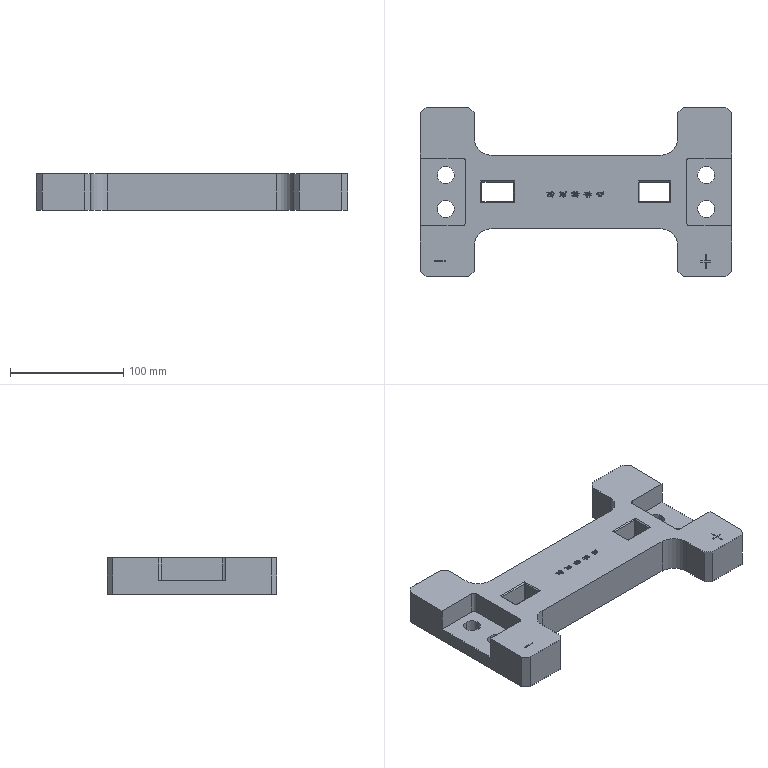NC program | NX | posted with a generic post | part box 275 x 150 x 32 mm
Lines 9668 to 10049 of 10049:
(DRILLING_COPY_1_COPY_1 , TOOL : ZXZ)
N19328 T01 M6
N19330 G54
N19332 G17 G0 G90 X-115. Y-15. S5000 M3
N19334 G43 Z30. H1
N19336 G94 G81 G98 Z-20.8 F250. R-16.8
N19338 Y15.
N19340 X-69.5 Y0. Z-1. R3.
N19342 X69.5
N19344 X115. Y15. Z-20.8 R-16.8
N19346 Y-15.
N19348 G80
N19350 G0 X115. Y-15. Z30.
N19352 M5
(FLOOR_WALL_1_1_COPY , TOOL : D10JING)
N19354 T11 M6
N19356 G54
N19358 G17 G0 G90 X-143. Y-23.634 S7000 M3
N19360 G43 Z30. H11
N19362 Z-18.8
N19364 G94 G1 Z-19.8 F1000.
N19366 X-142.
N19368 G3 X-142.5 Y-24.5 R1.
N19370 G1 Y24.5
N19372 X-137.562
N19374 Y-24.5
N19376 X-132.625
N19378 Y24.5
N19380 X-127.687
N19382 Y-24.5
N19384 X-122.75
N19386 Y24.5
N19388 X-117.813
N19390 Y-24.5
N19392 X-112.875
N19394 Y24.5
N19396 X-107.938
N19398 Y-24.5
N19400 X-103.
N19402 Y24.5
N19404 G3 X-103.25 Y24.433 R0.5
N19406 G1 Z-18.8
N19408 G0 Z30.
N19410 X-143.366 Y-24.5
N19412 Z-18.8
N19414 G1 Z-19.8
N19416 G3 X-142.5 Y-25. R1.
N19418 G1 X-102.5
N19420 Y25.
N19422 X-142.5
N19424 G3 X-143.366 Y24.5 R1.
N19426 G1 Z-18.8
N19428 G0 Z30.
N19430 X143. Y23.634
N19432 Z-18.8
N19434 G1 Z-19.8
N19436 X142.
N19438 G3 X142.5 Y24.5 R1.
N19440 G1 Y-24.5
N19442 X137.562
N19444 Y24.5
N19446 X132.625
N19448 Y-24.5
N19450 X127.687
N19452 Y24.5
N19454 X122.75
N19456 Y-24.5
N19458 X117.813
N19460 Y24.5
N19462 X112.875
N19464 Y-24.5
N19466 X107.938
N19468 Y24.5
N19470 X103.
N19472 Y-24.5
N19474 G3 X103.25 Y-24.433 R0.5
N19476 G1 Z-18.8
N19478 G0 Z30.
N19480 X143.366 Y24.5
N19482 Z-18.8
N19484 G1 Z-19.8
N19486 G3 X142.5 Y25. R1.
N19488 G1 X102.5
N19490 Y-25.
N19492 X142.5
N19494 G3 X143.366 Y-24.5 R1.
N19496 G1 Z-18.8
N19498 G0 Z30.
(ZLEVEL_PROFILE_1_COPY_COPY , TOOL : D10JING)
N19500 X-136.193 Y-81.161 S7500
N19502 Z-14.925
N19504 G1 Z-15.925 F1250.
N19506 X-135.527 Y-80.211
N19508 G3 X-135.639 Y-78.93 R1.
N19510 G1 X-138.3 Y-76.271
N19512 X-141.036 Y-73.536
N19514 X-141.43 Y-73.139
N19516 G3 X-142.711 Y-73.024 R1.
N19518 G1 X-143.665 Y-73.688
N19520 Z-14.925
N19522 G0 Z30.
N19524 X-136.194 Y-81.164
N19526 Z-30.85
N19528 G1 Z-31.85
N19530 X-135.528 Y-80.212
N19532 G3 X-135.64 Y-78.931 R1.
N19534 G1 X-138.3 Y-76.271
N19536 X-141.036 Y-73.536
N19538 X-141.431 Y-73.14
N19540 G3 X-142.712 Y-73.027 R1.
N19542 G1 X-143.664 Y-73.694
N19544 Z-30.85
N19546 G0 Z30.
N19548 X-143.662 Y73.693
N19550 Z-14.925
N19552 G1 Z-15.925
N19554 X-142.711 Y73.027
N19556 G3 X-141.43 Y73.139 R1.
N19558 G1 X-139.64 Y74.931
N19560 X-136.036 Y78.536
N19562 X-135.639 Y78.93
N19564 G3 X-135.524 Y80.211 R1.
N19566 G1 X-136.188 Y81.165
N19568 Z-14.925
N19570 G0 Z30.
N19572 X-143.664 Y73.694
N19574 Z-30.85
N19576 G1 Z-31.85
N19578 X-142.712 Y73.028
N19580 G3 X-141.431 Y73.14 R1.
N19582 G1 X-139.64 Y74.931
N19584 X-136.036 Y78.536
N19586 X-135.64 Y78.931
N19588 G3 X-135.527 Y80.212 R1.
N19590 G1 X-136.194 Y81.164
N19592 Z-30.85
N19594 G0 Z30.
N19596 X-91.669 Y81.429
N19598 Z-14.925
N19600 G1 Z-15.925
N19602 X-92.296 Y80.53
N19604 G3 X-92.181 Y79.249 R1.
N19606 G1 X-91.49 Y78.561
N19608 X-87.043 Y74.114
N19610 X-86.994 Y74.073
N19612 X-87.039 Y74.029
N19614 G2 X-85. Y70. R5.
N19616 G1 Y47.5
N19618 G3 X-75. Y37.5 R10.
N19620 G1 X75.
N19622 G3 X85. Y47.5 R10.
N19624 G1 Y70.
N19626 G2 X86.891 Y73.916 R5.
N19628 G1 X86.907 Y73.971
N19630 X87.172 Y74.243
N19632 X91.464 Y78.536
N19634 X92.181 Y79.249
N19636 G3 X92.296 Y80.53 R1.
N19638 G1 X91.672 Y81.425
N19640 Z-14.925
N19642 G0 Z30.
N19644 X-91.665 Y81.428
N19646 Z-30.85
N19648 G1 Z-31.85
N19650 X-92.293 Y80.532
N19652 G3 X-92.18 Y79.251 R1.
N19654 G1 X-91.49 Y78.561
N19656 X-87.042 Y74.113
N19658 X-86.994 Y74.073
N19660 X-87.039 Y74.029
N19662 G2 X-85. Y70. R5.
N19664 G1 Y47.5
N19666 G3 X-75. Y37.5 R10.
N19668 G1 X75.
N19670 G3 X85. Y47.5 R10.
N19672 G1 Y70.
N19674 G2 X86.891 Y73.916 R5.
N19676 G1 X86.906 Y73.972
N19678 X87.172 Y74.243
N19680 X91.464 Y78.536
N19682 X92.18 Y79.251
N19684 G3 X92.293 Y80.532 R1.
N19686 G1 X91.668 Y81.424
N19688 Z-30.85
N19690 G0 Z30.
N19692 X91.665 Y-81.426
N19694 Z-14.925
N19696 G1 Z-15.925
N19698 X92.293 Y-80.53
N19700 G3 X92.181 Y-79.249 R1.
N19702 G1 X89.77 Y-76.841
N19704 X86.464 Y-73.536
N19706 G2 X85. Y-70. R5.
N19708 G1 Y-47.5
N19710 G3 X75. Y-37.5 R10.
N19712 G1 X-75.
N19714 G3 X-85. Y-47.5 R10.
N19716 G1 Y-70.
N19718 G2 X-86.464 Y-73.536 R5.
N19720 G1 X-89.804 Y-76.871
N19722 X-92.181 Y-79.249
N19724 G3 X-92.293 Y-80.53 R1.
N19726 G1 X-91.668 Y-81.422
N19728 Z-14.925
N19730 G0 Z30.
N19732 X91.665 Y-81.428
N19734 Z-30.85
N19736 G1 Z-31.85
N19738 X92.292 Y-80.532
N19740 G3 X92.18 Y-79.251 R1.
N19742 G1 X89.77 Y-76.841
N19744 X86.464 Y-73.536
N19746 G2 X85. Y-70. R5.
N19748 G1 Y-47.5
N19750 G3 X75. Y-37.5 R10.
N19752 G1 X-75.
N19754 G3 X-85. Y-47.5 R10.
N19756 G1 Y-70.
N19758 G2 X-86.464 Y-73.536 R5.
N19760 G1 X-89.77 Y-76.841
N19762 X-92.18 Y-79.251
N19764 G3 X-92.292 Y-80.532 R1.
N19766 G1 X-91.668 Y-81.424
N19768 Z-30.85
N19770 G0 Z30.
N19772 X143.919 Y-73.34
N19774 Z-14.925
N19776 G1 Z-15.925
N19778 X143.02 Y-72.713
N19780 G3 X141.74 Y-72.828 R1.
N19782 G1 X141.06 Y-73.511
N19784 X138.273 Y-76.294
N19786 X135.639 Y-78.93
N19788 G3 X135.527 Y-80.211 R1.
N19790 G1 X136.193 Y-81.161
N19792 Z-14.925
N19794 G0 Z30.
N19796 X143.918 Y-73.344
N19798 Z-30.85
N19800 G1 Z-31.85
N19802 X143.022 Y-72.717
N19804 G3 X141.741 Y-72.83 R1.
N19806 G1 X141.06 Y-73.511
N19808 X138.3 Y-76.271
N19810 X135.64 Y-78.931
N19812 G3 X135.528 Y-80.212 R1.
N19814 G1 X136.194 Y-81.164
N19816 Z-30.85
N19818 G0 Z30.
N19820 X135.84 Y81.419
N19822 Z-14.925
N19824 G1 Z-15.925
N19826 X135.213 Y80.52
N19828 G3 X135.328 Y79.24 R1.
N19830 G1 X136.011 Y78.56
N19832 X139.664 Y74.904
N19834 X140.659 Y73.91
N19836 X140.658 Y73.876
N19838 G2 X141.543 Y72.942 R5.
N19840 X141.74 Y72.828 R0.139
N19842 G3 X143.02 Y72.717 R1.
N19844 G1 X143.914 Y73.343
N19846 Z-14.925
N19848 G0 Z30.
N19850 X135.844 Y81.418
N19852 Z-30.85
N19854 G1 Z-31.85
N19856 X135.217 Y80.522
N19858 G3 X135.33 Y79.241 R1.
N19860 G1 X136.011 Y78.56
N19862 X139.64 Y74.931
N19864 X140.659 Y73.911
N19866 X140.658 Y73.876
N19868 G2 X141.524 Y72.968 R5.
N19870 X141.741 Y72.83 R0.196
N19872 G3 X143.022 Y72.718 R1.
N19874 G1 X143.915 Y73.344
N19876 Z-30.85
N19878 G0 Z30.
N19880 M5
(ZLEVEL_PROFILE_1_COPY_1_COPY , TOOL : D6A45)
N19882 T22 M6
N19884 G54
N19886 G17 G0 G90 X76.065 Y-34.703 S7500 M3
N19888 G43 Z30. H22
N19890 Z0.
N19892 G94 G1 Z-1. F1000.
N19894 X75.52 Y-33.759
N19896 G3 X75. Y-33.459 R0.6
N19898 G1 X-75.
N19900 G3 X-89.041 Y-47.5 R14.041
N19902 G1 Y-70.001
N19904 G2 X-89.321 Y-70.677 R0.994
N19906 G1 X-94.323 Y-75.678
N19908 G2 X-94.999 Y-75.959 R0.957
N19910 G1 X-132.501
N19912 G2 X-133.177 Y-75.678 R0.957
N19914 G1 X-138.178 Y-70.677
N19916 G2 X-138.459 Y-70.001 R0.956
N19918 G1 Y-29.999
N19920 G2 X-137.501 Y-29.041 R0.958
N19922 G1 X-100.5
N19924 G3 X-98.459 Y-27. R2.041
N19926 G1 Y27.
N19928 G3 X-100.5 Y29.041 R2.041
N19930 G1 X-137.501
N19932 G2 X-138.459 Y29.999 R0.958
N19934 G1 Y70.001
N19936 G2 X-138.178 Y70.677 R0.956
N19938 G1 X-133.177 Y75.678
N19940 G2 X-132.501 Y75.959 R0.957
N19942 G1 X-94.999
N19944 G2 X-94.323 Y75.678 R0.957
N19946 G1 X-89.319 Y70.675
N19948 G2 X-89.041 Y70.001 R0.994
N19950 G1 Y47.5
N19952 G3 X-75. Y33.459 R14.041
N19954 G1 X75.
N19956 G3 X89.041 Y47.5 R14.041
N19958 G1 Y70.001
N19960 G2 X89.322 Y70.677 R0.994
N19962 G1 X94.323 Y75.678
N19964 G2 X94.999 Y75.959 R0.957
N19966 G1 X132.501
N19968 G2 X133.177 Y75.678 R0.957
N19970 G1 X138.178 Y70.677
N19972 G2 X138.459 Y70.001 R0.956
N19974 G1 Y29.999
N19976 G2 X137.501 Y29.041 R0.958
N19978 G1 X100.5
N19980 G3 X98.459 Y27. R2.041
N19982 G1 Y-27.
N19984 G3 X100.5 Y-29.041 R2.041
N19986 G1 X137.501
N19988 G2 X138.459 Y-29.999 R0.958
N19990 G1 Y-70.001
N19992 G2 X138.178 Y-70.677 R0.956
N19994 G1 X133.177 Y-75.678
N19996 G2 X132.501 Y-75.959 R0.957
N19998 G1 X94.999
N20000 G2 X94.323 Y-75.678 R0.957
N20002 G1 X89.322 Y-70.677
N20004 G2 X89.041 Y-70.001 R0.994
N20006 G1 Y-47.5
N20008 G3 X75. Y-33.459 R14.041
N20010 X74.48 Y-33.759 R0.6
N20012 G1 X73.961 Y-34.659
N20014 Z0.
N20016 G0 Z30.
(ZLEVEL_PROFILE_1_COPY_1_COPY_COPY , TOOL : D6A45)
N20018 X139.745 Y26.533
N20020 Z-19.8
N20022 G1 Z-20.8
N20024 X139.057 Y27.
N20026 G3 X138.459 Y27.043 R0.6
N20028 G1 Y-27.043
N20030 G3 X139.055 Y-26.979 R0.6
N20032 G1 X139.7 Y-26.509
N20034 Z-19.8
N20036 G0 Z30.
N20038 X-139.701 Y-26.511
N20040 Z-19.8
N20042 G1 Z-20.8
N20044 X-139.055 Y-26.98
N20046 G3 X-138.459 Y-27.043 R0.6
N20048 G1 Y27.043
N20050 G3 X-139.055 Y26.979 R0.6
N20052 G1 X-139.698 Y26.509
N20054 Z-19.8
N20056 G0 Z30.
N20058 M5
N20060 M2